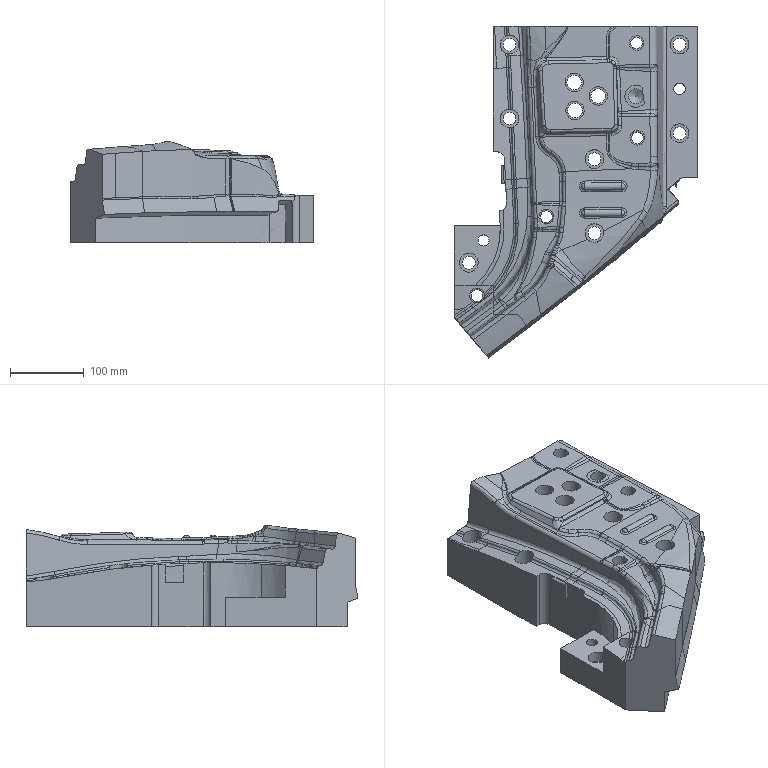Part | NX | features solid 2 | 1 solid | 385 faces | box 330 x 448.974 x 137.333 mm | volume 9318312 mm3 | spline 311 | plane 38 | cylinder 35 | cone 1 | commonest cylinder face diameters 20 x11 17.5 x7 25.5 x7 16 x5 25 x3 15 x1